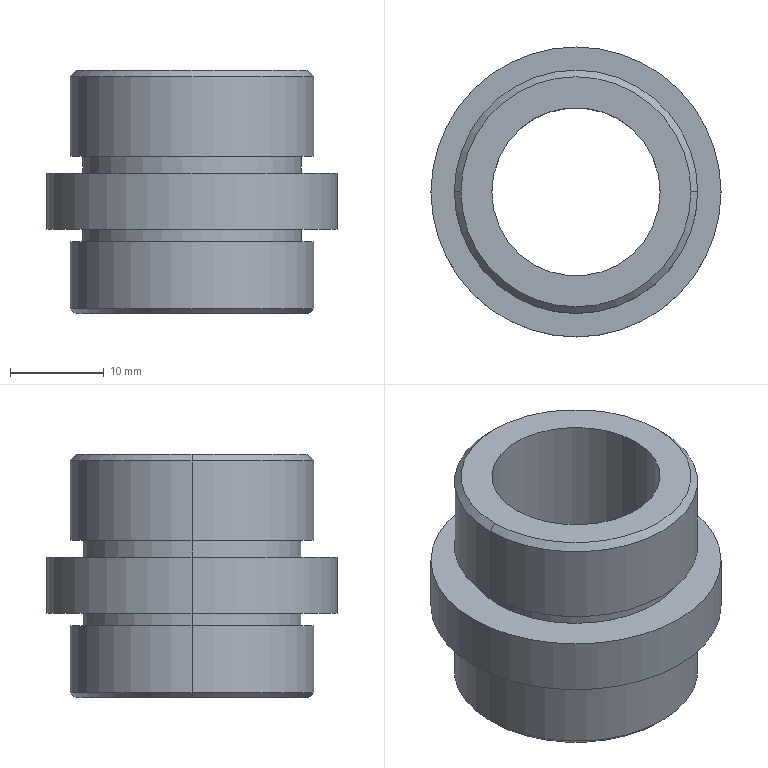Part | STEP file | 32 | 1 solid | 24 faces | box 31 x 31 x 26 mm | volume 8159 mm3 | cylinder 12 | cone 6 | plane 6 | commonest cylinder face diameters 23.4 x4 26 x4 18 x2 31 x2